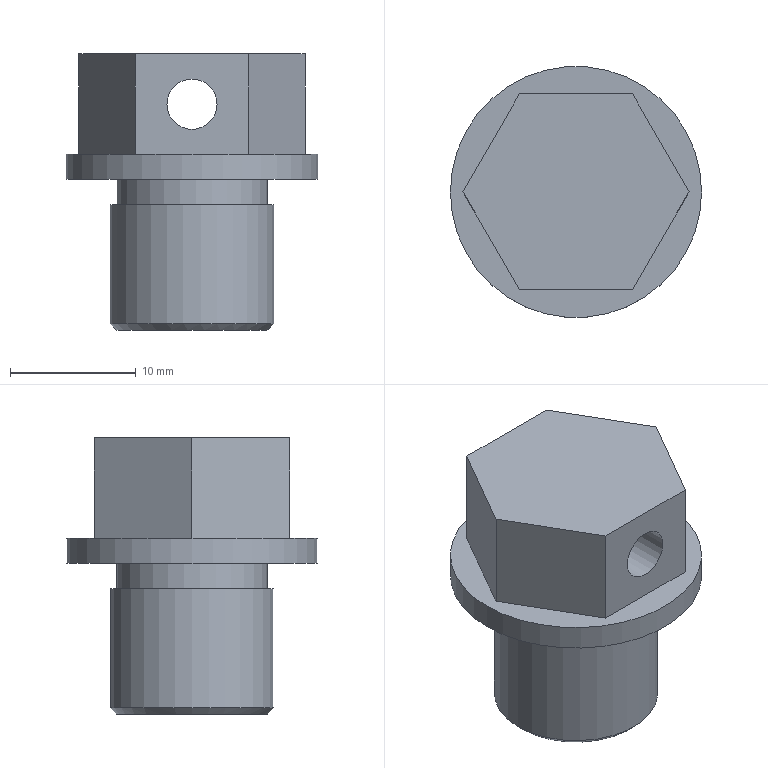Part | NX | features DATUM_CSYS 6, EXTRUDE 5, SKETCH 5, CHAMFER 1 | 1 solid | 16 faces | box 20 x 20 x 22 mm | volume 3665 mm3 | plane 11 | cylinder 4 | cone 1 | commonest cylinder face diameters 4 x1 12 x1 13 x1 20 x1
STEP:
#1=CARTESIAN_POINT('',(-9.,0.,0.));
#2=VERTEX_POINT('',#1);
#3=CARTESIAN_POINT('',(-4.5,-7.794,0.));
#4=VERTEX_POINT('',#3);
#5=CARTESIAN_POINT('',(-9.,0.,0.));
#6=DIRECTION('',(0.5,-0.866,0.));
#7=VECTOR('',#6,1000.);
#8=LINE('',#5,#7);
#9=EDGE_CURVE('',#2,#4,#8,.T.);
#10=ORIENTED_EDGE('',*,*,#9,.T.);
#11=CARTESIAN_POINT('',(-4.5,-7.794,8.));
#12=VERTEX_POINT('',#11);
#13=CARTESIAN_POINT('',(-4.5,-7.794,8.));
#14=DIRECTION('',(0.,0.,-1.));
#15=VECTOR('',#14,1000.);
#16=LINE('',#13,#15);
#17=EDGE_CURVE('',#12,#4,#16,.T.);
#18=ORIENTED_EDGE('',*,*,#17,.F.);
#19=CARTESIAN_POINT('',(-9.,0.,8.));
#20=VERTEX_POINT('',#19);
#21=CARTESIAN_POINT('',(-9.,0.,8.));
#22=DIRECTION('',(0.5,-0.866,0.));
#23=VECTOR('',#22,1000.);
#24=LINE('',#21,#23);
#25=EDGE_CURVE('',#20,#12,#24,.T.);
#26=ORIENTED_EDGE('',*,*,#25,.F.);
#27=CARTESIAN_POINT('',(-9.,0.,8.));
#28=DIRECTION('',(0.,0.,-1.));
#29=VECTOR('',#28,1000.);
#30=LINE('',#27,#29);
#31=EDGE_CURVE('',#20,#2,#30,.T.);
#32=ORIENTED_EDGE('',*,*,#31,.T.);
#33=EDGE_LOOP('',(#10,#18,#26,#32));
#34=FACE_BOUND('',#33,.T.);
#35=CARTESIAN_POINT('',(-9.,0.,8.));
#36=DIRECTION('',(0.866,0.5,0.));
#37=DIRECTION('',(-0.5,0.866,0.));
#38=AXIS2_PLACEMENT_3D('',#35,#36,#37);
#39=PLANE('',#38);
#40=ADVANCED_FACE('',(#34),#39,.F.);
#41=CARTESIAN_POINT('',(-2.,-7.794,4.));
#42=VERTEX_POINT('',#41);
#43=CARTESIAN_POINT('',(0.,-7.794,4.));
#44=DIRECTION('',(0.,1.,0.));
#45=DIRECTION('',(-1.,0.,0.));
#46=AXIS2_PLACEMENT_3D('',#43,#44,#45);
#47=CIRCLE('',#46,2.);
#48=EDGE_CURVE('',#42,#42,#47,.F.);
#49=ORIENTED_EDGE('',*,*,#48,.F.);
#50=EDGE_LOOP('',(#49));
#51=FACE_BOUND('',#50,.T.);
#52=CARTESIAN_POINT('',(4.5,-7.794,0.));
#53=VERTEX_POINT('',#52);
#54=CARTESIAN_POINT('',(-4.5,-7.794,0.));
#55=DIRECTION('',(1.,0.,0.));
#56=VECTOR('',#55,1000.);
#57=LINE('',#54,#56);
#58=EDGE_CURVE('',#4,#53,#57,.T.);
#59=ORIENTED_EDGE('',*,*,#58,.T.);
#60=CARTESIAN_POINT('',(4.5,-7.794,8.));
#61=VERTEX_POINT('',#60);
#62=CARTESIAN_POINT('',(4.5,-7.794,8.));
#63=DIRECTION('',(0.,0.,-1.));
#64=VECTOR('',#63,1000.);
#65=LINE('',#62,#64);
#66=EDGE_CURVE('',#61,#53,#65,.T.);
#67=ORIENTED_EDGE('',*,*,#66,.F.);
#68=CARTESIAN_POINT('',(-4.5,-7.794,8.));
#69=DIRECTION('',(1.,0.,0.));
#70=VECTOR('',#69,1000.);
#71=LINE('',#68,#70);
#72=EDGE_CURVE('',#12,#61,#71,.T.);
#73=ORIENTED_EDGE('',*,*,#72,.F.);
#74=ORIENTED_EDGE('',*,*,#17,.T.);
#75=EDGE_LOOP('',(#59,#67,#73,#74));
#76=FACE_BOUND('',#75,.T.);
#77=CARTESIAN_POINT('',(-4.5,-7.794,8.));
#78=DIRECTION('',(0.,1.,0.));
#79=DIRECTION('',(-1.,0.,0.));
#80=AXIS2_PLACEMENT_3D('',#77,#78,#79);
#81=PLANE('',#80);
#82=ADVANCED_FACE('',(#51,#76),#81,.F.);
#83=CARTESIAN_POINT('',(9.,0.,0.));
#84=VERTEX_POINT('',#83);
#85=CARTESIAN_POINT('',(4.5,-7.794,0.));
#86=DIRECTION('',(0.5,0.866,0.));
#87=VECTOR('',#86,1000.);
#88=LINE('',#85,#87);
#89=EDGE_CURVE('',#53,#84,#88,.T.);
#90=ORIENTED_EDGE('',*,*,#89,.T.);
#91=CARTESIAN_POINT('',(9.,0.,8.));
#92=VERTEX_POINT('',#91);
#93=CARTESIAN_POINT('',(9.,0.,8.));
#94=DIRECTION('',(0.,0.,-1.));
#95=VECTOR('',#94,1000.);
#96=LINE('',#93,#95);
#97=EDGE_CURVE('',#92,#84,#96,.T.);
#98=ORIENTED_EDGE('',*,*,#97,.F.);
#99=CARTESIAN_POINT('',(4.5,-7.794,8.));
#100=DIRECTION('',(0.5,0.866,0.));
#101=VECTOR('',#100,1000.);
#102=LINE('',#99,#101);
#103=EDGE_CURVE('',#61,#92,#102,.T.);
#104=ORIENTED_EDGE('',*,*,#103,.F.);
#105=ORIENTED_EDGE('',*,*,#66,.T.);
#106=EDGE_LOOP('',(#90,#98,#104,#105));
#107=FACE_BOUND('',#106,.T.);
#108=CARTESIAN_POINT('',(4.5,-7.794,8.));
#109=DIRECTION('',(-0.866,0.5,0.));
#110=DIRECTION('',(-0.5,-0.866,0.));
#111=AXIS2_PLACEMENT_3D('',#108,#109,#110);
#112=PLANE('',#111);
#113=ADVANCED_FACE('',(#107),#112,.F.);
#114=CARTESIAN_POINT('',(4.5,7.794,0.));
#115=VERTEX_POINT('',#114);
#116=CARTESIAN_POINT('',(9.,0.,0.));
#117=DIRECTION('',(-0.5,0.866,0.));
#118=VECTOR('',#117,1000.);
#119=LINE('',#116,#118);
#120=EDGE_CURVE('',#84,#115,#119,.T.);
#121=ORIENTED_EDGE('',*,*,#120,.T.);
#122=CARTESIAN_POINT('',(4.5,7.794,8.));
#123=VERTEX_POINT('',#122);
#124=CARTESIAN_POINT('',(4.5,7.794,8.));
#125=DIRECTION('',(0.,0.,-1.));
#126=VECTOR('',#125,1000.);
#127=LINE('',#124,#126);
#128=EDGE_CURVE('',#123,#115,#127,.T.);
#129=ORIENTED_EDGE('',*,*,#128,.F.);
#130=CARTESIAN_POINT('',(9.,0.,8.));
#131=DIRECTION('',(-0.5,0.866,0.));
#132=VECTOR('',#131,1000.);
#133=LINE('',#130,#132);
#134=EDGE_CURVE('',#92,#123,#133,.T.);
#135=ORIENTED_EDGE('',*,*,#134,.F.);
#136=ORIENTED_EDGE('',*,*,#97,.T.);
#137=EDGE_LOOP('',(#121,#129,#135,#136));
#138=FACE_BOUND('',#137,.T.);
#139=CARTESIAN_POINT('',(9.,0.,8.));
#140=DIRECTION('',(-0.866,-0.5,0.));
#141=DIRECTION('',(0.5,-0.866,0.));
#142=AXIS2_PLACEMENT_3D('',#139,#140,#141);
#143=PLANE('',#142);
#144=ADVANCED_FACE('',(#138),#143,.F.);
#145=CARTESIAN_POINT('',(2.,7.794,4.));
#146=VERTEX_POINT('',#145);
#147=CARTESIAN_POINT('',(0.,7.794,4.));
#148=DIRECTION('',(0.,-1.,0.));
#149=DIRECTION('',(1.,0.,0.));
#150=AXIS2_PLACEMENT_3D('',#147,#148,#149);
#151=CIRCLE('',#150,2.);
#152=EDGE_CURVE('',#146,#146,#151,.F.);
#153=ORIENTED_EDGE('',*,*,#152,.F.);
#154=EDGE_LOOP('',(#153));
#155=FACE_BOUND('',#154,.T.);
#156=CARTESIAN_POINT('',(-4.5,7.794,0.));
#157=VERTEX_POINT('',#156);
#158=CARTESIAN_POINT('',(4.5,7.794,0.));
#159=DIRECTION('',(-1.,0.,0.));
#160=VECTOR('',#159,1000.);
#161=LINE('',#158,#160);
#162=EDGE_CURVE('',#115,#157,#161,.T.);
#163=ORIENTED_EDGE('',*,*,#162,.T.);
#164=CARTESIAN_POINT('',(-4.5,7.794,8.));
#165=VERTEX_POINT('',#164);
#166=CARTESIAN_POINT('',(-4.5,7.794,8.));
#167=DIRECTION('',(0.,0.,-1.));
#168=VECTOR('',#167,1000.);
#169=LINE('',#166,#168);
#170=EDGE_CURVE('',#165,#157,#169,.T.);
#171=ORIENTED_EDGE('',*,*,#170,.F.);
#172=CARTESIAN_POINT('',(4.5,7.794,8.));
#173=DIRECTION('',(-1.,0.,0.));
#174=VECTOR('',#173,1000.);
#175=LINE('',#172,#174);
#176=EDGE_CURVE('',#123,#165,#175,.T.);
#177=ORIENTED_EDGE('',*,*,#176,.F.);
#178=ORIENTED_EDGE('',*,*,#128,.T.);
#179=EDGE_LOOP('',(#163,#171,#177,#178));
#180=FACE_BOUND('',#179,.T.);
#181=CARTESIAN_POINT('',(4.5,7.794,8.));
#182=DIRECTION('',(0.,-1.,0.));
#183=DIRECTION('',(1.,0.,0.));
#184=AXIS2_PLACEMENT_3D('',#181,#182,#183);
#185=PLANE('',#184);
#186=ADVANCED_FACE('',(#155,#180),#185,.F.);
#187=CARTESIAN_POINT('',(-4.5,7.794,0.));
#188=DIRECTION('',(-0.5,-0.866,0.));
#189=VECTOR('',#188,1000.);
#190=LINE('',#187,#189);
#191=EDGE_CURVE('',#157,#2,#190,.T.);
#192=ORIENTED_EDGE('',*,*,#191,.T.);
#193=ORIENTED_EDGE('',*,*,#31,.F.);
#194=CARTESIAN_POINT('',(-4.5,7.794,8.));
#195=DIRECTION('',(-0.5,-0.866,0.));
#196=VECTOR('',#195,1000.);
#197=LINE('',#194,#196);
#198=EDGE_CURVE('',#165,#20,#197,.T.);
#199=ORIENTED_EDGE('',*,*,#198,.F.);
#200=ORIENTED_EDGE('',*,*,#170,.T.);
#201=EDGE_LOOP('',(#192,#193,#199,#200));
#202=FACE_BOUND('',#201,.T.);
#203=CARTESIAN_POINT('',(-4.5,7.794,8.));
#204=DIRECTION('',(0.866,-0.5,0.));
#205=DIRECTION('',(0.5,0.866,0.));
#206=AXIS2_PLACEMENT_3D('',#203,#204,#205);
#207=PLANE('',#206);
#208=ADVANCED_FACE('',(#202),#207,.F.);
#209=ORIENTED_EDGE('',*,*,#25,.T.);
#210=ORIENTED_EDGE('',*,*,#72,.T.);
#211=ORIENTED_EDGE('',*,*,#103,.T.);
#212=ORIENTED_EDGE('',*,*,#134,.T.);
#213=ORIENTED_EDGE('',*,*,#176,.T.);
#214=ORIENTED_EDGE('',*,*,#198,.T.);
#215=EDGE_LOOP('',(#209,#210,#211,#212,#213,#214));
#216=FACE_BOUND('',#215,.T.);
#217=CARTESIAN_POINT('',(0.,0.,8.));
#218=DIRECTION('',(0.,0.,1.));
#219=DIRECTION('',(1.,0.,0.));
#220=AXIS2_PLACEMENT_3D('',#217,#218,#219);
#221=PLANE('',#220);
#222=ADVANCED_FACE('',(#216),#221,.T.);
#223=CARTESIAN_POINT('',(10.,0.,0.));
#224=VERTEX_POINT('',#223);
#225=CARTESIAN_POINT('',(0.,0.,0.));
#226=DIRECTION('',(0.,0.,1.));
#227=DIRECTION('',(1.,0.,0.));
#228=AXIS2_PLACEMENT_3D('',#225,#226,#227);
#229=CIRCLE('',#228,10.);
#230=EDGE_CURVE('',#224,#224,#229,.T.);
#231=ORIENTED_EDGE('',*,*,#230,.T.);
#232=EDGE_LOOP('',(#231));
#233=FACE_BOUND('',#232,.T.);
#234=ORIENTED_EDGE('',*,*,#9,.F.);
#235=ORIENTED_EDGE('',*,*,#191,.F.);
#236=ORIENTED_EDGE('',*,*,#162,.F.);
#237=ORIENTED_EDGE('',*,*,#120,.F.);
#238=ORIENTED_EDGE('',*,*,#89,.F.);
#239=ORIENTED_EDGE('',*,*,#58,.F.);
#240=EDGE_LOOP('',(#234,#235,#236,#237,#238,#239));
#241=FACE_BOUND('',#240,.T.);
#242=CARTESIAN_POINT('',(0.,0.,0.));
#243=DIRECTION('',(0.,0.,1.));
#244=DIRECTION('',(1.,0.,0.));
#245=AXIS2_PLACEMENT_3D('',#242,#243,#244);
#246=PLANE('',#245);
#247=ADVANCED_FACE('',(#233,#241),#246,.T.);
#248=CARTESIAN_POINT('',(10.,0.,-2.));
#249=VERTEX_POINT('',#248);
#250=CARTESIAN_POINT('',(0.,0.,-2.));
#251=DIRECTION('',(0.,0.,1.));
#252=DIRECTION('',(1.,0.,0.));
#253=AXIS2_PLACEMENT_3D('',#250,#251,#252);
#254=CIRCLE('',#253,10.);
#255=EDGE_CURVE('',#249,#249,#254,.T.);
#256=ORIENTED_EDGE('',*,*,#255,.T.);
#257=EDGE_LOOP('',(#256));
#258=FACE_BOUND('',#257,.T.);
#259=ORIENTED_EDGE('',*,*,#230,.F.);
#260=EDGE_LOOP('',(#259));
#261=FACE_BOUND('',#260,.T.);
#262=CARTESIAN_POINT('',(0.,0.,-2.));
#263=DIRECTION('',(0.,0.,1.));
#264=DIRECTION('',(1.,0.,0.));
#265=AXIS2_PLACEMENT_3D('',#262,#263,#264);
#266=CYLINDRICAL_SURFACE('',#265,10.);
#267=ADVANCED_FACE('',(#258,#261),#266,.T.);
#268=CARTESIAN_POINT('',(6.,0.,-2.));
#269=VERTEX_POINT('',#268);
#270=CARTESIAN_POINT('',(0.,0.,-2.));
#271=DIRECTION('',(0.,0.,-1.));
#272=DIRECTION('',(1.,0.,0.));
#273=AXIS2_PLACEMENT_3D('',#270,#271,#272);
#274=CIRCLE('',#273,6.);
#275=EDGE_CURVE('',#269,#269,#274,.T.);
#276=ORIENTED_EDGE('',*,*,#275,.F.);
#277=EDGE_LOOP('',(#276));
#278=FACE_BOUND('',#277,.T.);
#279=ORIENTED_EDGE('',*,*,#255,.F.);
#280=EDGE_LOOP('',(#279));
#281=FACE_BOUND('',#280,.T.);
#282=CARTESIAN_POINT('',(0.,0.,-2.));
#283=DIRECTION('',(0.,0.,1.));
#284=DIRECTION('',(1.,0.,0.));
#285=AXIS2_PLACEMENT_3D('',#282,#283,#284);
#286=PLANE('',#285);
#287=ADVANCED_FACE('',(#278,#281),#286,.F.);
#288=CARTESIAN_POINT('',(6.,0.,-4.));
#289=VERTEX_POINT('',#288);
#290=CARTESIAN_POINT('',(0.,0.,-4.));
#291=DIRECTION('',(0.,0.,-1.));
#292=DIRECTION('',(1.,0.,0.));
#293=AXIS2_PLACEMENT_3D('',#290,#291,#292);
#294=CIRCLE('',#293,6.);
#295=EDGE_CURVE('',#289,#289,#294,.T.);
#296=ORIENTED_EDGE('',*,*,#295,.F.);
#297=EDGE_LOOP('',(#296));
#298=FACE_BOUND('',#297,.T.);
#299=ORIENTED_EDGE('',*,*,#275,.T.);
#300=EDGE_LOOP('',(#299));
#301=FACE_BOUND('',#300,.T.);
#302=CARTESIAN_POINT('',(0.,0.,-4.));
#303=DIRECTION('',(0.,0.,1.));
#304=DIRECTION('',(1.,0.,0.));
#305=AXIS2_PLACEMENT_3D('',#302,#303,#304);
#306=CYLINDRICAL_SURFACE('',#305,6.);
#307=ADVANCED_FACE('',(#298,#301),#306,.T.);
#308=CARTESIAN_POINT('',(-6.5,0.,-13.5));
#309=VERTEX_POINT('',#308);
#310=CARTESIAN_POINT('',(0.,0.,-13.5));
#311=DIRECTION('',(0.,0.,-1.));
#312=DIRECTION('',(-1.,0.,0.));
#313=AXIS2_PLACEMENT_3D('',#310,#311,#312);
#314=CIRCLE('',#313,6.5);
#315=EDGE_CURVE('',#309,#309,#314,.F.);
#316=ORIENTED_EDGE('',*,*,#315,.T.);
#317=EDGE_LOOP('',(#316));
#318=FACE_BOUND('',#317,.T.);
#319=CARTESIAN_POINT('',(6.5,0.,-4.));
#320=VERTEX_POINT('',#319);
#321=CARTESIAN_POINT('',(0.,0.,-4.));
#322=DIRECTION('',(0.,0.,-1.));
#323=DIRECTION('',(1.,0.,0.));
#324=AXIS2_PLACEMENT_3D('',#321,#322,#323);
#325=CIRCLE('',#324,6.5);
#326=EDGE_CURVE('',#320,#320,#325,.T.);
#327=ORIENTED_EDGE('',*,*,#326,.T.);
#328=EDGE_LOOP('',(#327));
#329=FACE_BOUND('',#328,.T.);
#330=CARTESIAN_POINT('',(0.,0.,-14.));
#331=DIRECTION('',(0.,0.,1.));
#332=DIRECTION('',(1.,0.,0.));
#333=AXIS2_PLACEMENT_3D('',#330,#331,#332);
#334=CYLINDRICAL_SURFACE('',#333,6.5);
#335=ADVANCED_FACE('',(#318,#329),#334,.T.);
#336=CARTESIAN_POINT('',(-6.,0.,-14.));
#337=VERTEX_POINT('',#336);
#338=CARTESIAN_POINT('',(0.,0.,-14.));
#339=DIRECTION('',(0.,0.,-1.));
#340=DIRECTION('',(-1.,0.,0.));
#341=AXIS2_PLACEMENT_3D('',#338,#339,#340);
#342=CIRCLE('',#341,6.);
#343=EDGE_CURVE('',#337,#337,#342,.T.);
#344=ORIENTED_EDGE('',*,*,#343,.T.);
#345=EDGE_LOOP('',(#344));
#346=FACE_BOUND('',#345,.T.);
#347=CARTESIAN_POINT('',(0.,0.,-14.));
#348=DIRECTION('',(0.,0.,-1.));
#349=DIRECTION('',(-1.,0.,0.));
#350=AXIS2_PLACEMENT_3D('',#347,#348,#349);
#351=PLANE('',#350);
#352=ADVANCED_FACE('',(#346),#351,.T.);
#353=ORIENTED_EDGE('',*,*,#295,.T.);
#354=EDGE_LOOP('',(#353));
#355=FACE_BOUND('',#354,.T.);
#356=ORIENTED_EDGE('',*,*,#326,.F.);
#357=EDGE_LOOP('',(#356));
#358=FACE_BOUND('',#357,.T.);
#359=CARTESIAN_POINT('',(0.,0.,-4.));
#360=DIRECTION('',(0.,0.,-1.));
#361=DIRECTION('',(-1.,0.,0.));
#362=AXIS2_PLACEMENT_3D('',#359,#360,#361);
#363=PLANE('',#362);
#364=ADVANCED_FACE('',(#355,#358),#363,.F.);
#365=ORIENTED_EDGE('',*,*,#152,.T.);
#366=EDGE_LOOP('',(#365));
#367=FACE_BOUND('',#366,.T.);
#368=ORIENTED_EDGE('',*,*,#48,.T.);
#369=EDGE_LOOP('',(#368));
#370=FACE_BOUND('',#369,.T.);
#371=CARTESIAN_POINT('',(0.,-12.5,4.));
#372=DIRECTION('',(0.,1.,0.));
#373=DIRECTION('',(0.,0.,1.));
#374=AXIS2_PLACEMENT_3D('',#371,#372,#373);
#375=CYLINDRICAL_SURFACE('',#374,2.);
#376=ADVANCED_FACE('',(#367,#370),#375,.F.);
#377=ORIENTED_EDGE('',*,*,#315,.F.);
#378=EDGE_LOOP('',(#377));
#379=FACE_BOUND('',#378,.T.);
#380=ORIENTED_EDGE('',*,*,#343,.F.);
#381=EDGE_LOOP('',(#380));
#382=FACE_BOUND('',#381,.T.);
#383=CARTESIAN_POINT('',(0.,0.,-14.));
#384=DIRECTION('',(0.,0.,1.));
#385=DIRECTION('',(1.,0.,0.));
#386=AXIS2_PLACEMENT_3D('',#383,#384,#385);
#387=CONICAL_SURFACE('',#386,6.,0.7854);
#388=ADVANCED_FACE('',(#379,#382),#387,.T.);
#389=CLOSED_SHELL('',(#40,#82,#113,#144,#186,#208,#222,#247,#267,#287,#307,#335,#352,#364,#376,#388));
#390=MANIFOLD_SOLID_BREP('',#389);
#391=(LENGTH_UNIT()NAMED_UNIT(*)SI_UNIT(.MILLI.,.METRE.));
#392=UNCERTAINTY_MEASURE_WITH_UNIT(LENGTH_MEASURE(0.00001),#391,'','');
#393=(NAMED_UNIT(*)PLANE_ANGLE_UNIT()SI_UNIT($,.RADIAN.));
#394=(NAMED_UNIT(*)SI_UNIT($,.STERADIAN.)SOLID_ANGLE_UNIT());
#395=(GEOMETRIC_REPRESENTATION_CONTEXT(3)GLOBAL_UNCERTAINTY_ASSIGNED_CONTEXT((#392))GLOBAL_UNIT_ASSIGNED_CONTEXT((#391,#393,#394))REPRESENTATION_CONTEXT('',''));
#396=ADVANCED_BREP_SHAPE_REPRESENTATION('',(#390),#395);